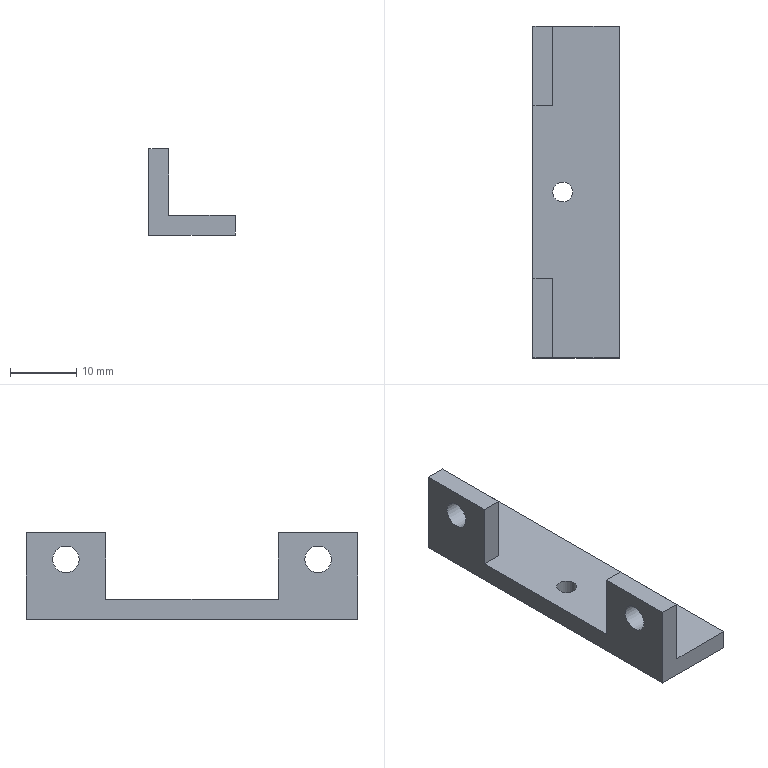Part | STEP file | 1-02 | 1 solid | 15 faces | box 13 x 50 x 13 mm | volume 2573 mm3 | plane 12 | cylinder 3 | commonest cylinder face diameters 4 x2 3 x1
STEP:
#1=CARTESIAN_POINT('',(0.,0.,0.));
#2=DIRECTION('',(0.,0.,1.));
#3=DIRECTION('',(1.,0.,0.));
#4=AXIS2_PLACEMENT_3D('',#1,#2,#3);
#5=CARTESIAN_POINT('',(-6.5,-25.,-3.));
#6=VERTEX_POINT('',#5);
#7=CARTESIAN_POINT('',(6.5,-25.,-3.));
#8=VERTEX_POINT('',#7);
#9=CARTESIAN_POINT('',(-6.5,-25.,-3.));
#10=DIRECTION('',(1.,0.,0.));
#11=VECTOR('',#10,1.);
#12=LINE('',#9,#11);
#13=CARTESIAN_POINT('',(18.5,0.,-3.));
#14=DIRECTION('',(0.,0.,1.));
#15=DIRECTION('',(1.,0.,0.));
#16=AXIS2_PLACEMENT_3D('',#13,#14,#15);
#17=PLANE('',#16);
#18=CARTESIAN_POINT('',(-25.,-25.));
#19=DIRECTION('',(1.,0.));
#20=VECTOR('',#19,1.);
#21=LINE('',#18,#20);
#22=(GEOMETRIC_REPRESENTATION_CONTEXT(2)PARAMETRIC_REPRESENTATION_CONTEXT()REPRESENTATION_CONTEXT('',''));
#23=DEFINITIONAL_REPRESENTATION('',(#21),#22);
#24=PCURVE('',#17,#23);
#25=CARTESIAN_POINT('',(0.,-25.,3.5));
#26=DIRECTION('',(0.,1.,0.));
#27=DIRECTION('',(1.,0.,0.));
#28=AXIS2_PLACEMENT_3D('',#25,#26,#27);
#29=PLANE('',#28);
#30=CARTESIAN_POINT('',(-6.5,6.5));
#31=DIRECTION('',(1.,0.));
#32=VECTOR('',#31,1.);
#33=LINE('',#30,#32);
#34=(GEOMETRIC_REPRESENTATION_CONTEXT(2)PARAMETRIC_REPRESENTATION_CONTEXT()REPRESENTATION_CONTEXT('',''));
#35=DEFINITIONAL_REPRESENTATION('',(#33),#34);
#36=PCURVE('',#29,#35);
#37=SURFACE_CURVE('',#12,(#24,#36),.PCURVE_S1.);
#38=EDGE_CURVE('',#6,#8,#37,.T.);
#39=ORIENTED_EDGE('',*,*,#38,.T.);
#40=CARTESIAN_POINT('',(6.5,25.,-3.));
#41=VERTEX_POINT('',#40);
#42=CARTESIAN_POINT('',(6.5,-25.,-3.));
#43=DIRECTION('',(0.,1.,0.));
#44=VECTOR('',#43,1.);
#45=LINE('',#42,#44);
#46=CARTESIAN_POINT('',(-12.,-25.));
#47=DIRECTION('',(0.,1.));
#48=VECTOR('',#47,1.);
#49=LINE('',#46,#48);
#50=(GEOMETRIC_REPRESENTATION_CONTEXT(2)PARAMETRIC_REPRESENTATION_CONTEXT()REPRESENTATION_CONTEXT('',''));
#51=DEFINITIONAL_REPRESENTATION('',(#49),#50);
#52=PCURVE('',#17,#51);
#53=CARTESIAN_POINT('',(6.5,0.,-1.5));
#54=DIRECTION('',(-1.,0.,0.));
#55=DIRECTION('',(0.,1.,0.));
#56=AXIS2_PLACEMENT_3D('',#53,#54,#55);
#57=PLANE('',#56);
#58=CARTESIAN_POINT('',(-25.,1.5));
#59=DIRECTION('',(1.,0.));
#60=VECTOR('',#59,1.);
#61=LINE('',#58,#60);
#62=(GEOMETRIC_REPRESENTATION_CONTEXT(2)PARAMETRIC_REPRESENTATION_CONTEXT()REPRESENTATION_CONTEXT('',''));
#63=DEFINITIONAL_REPRESENTATION('',(#61),#62);
#64=PCURVE('',#57,#63);
#65=SURFACE_CURVE('',#45,(#52,#64),.PCURVE_S1.);
#66=EDGE_CURVE('',#8,#41,#65,.T.);
#67=ORIENTED_EDGE('',*,*,#66,.T.);
#68=CARTESIAN_POINT('',(-6.5,25.,-3.));
#69=VERTEX_POINT('',#68);
#70=CARTESIAN_POINT('',(6.5,25.,-3.));
#71=DIRECTION('',(-1.,0.,0.));
#72=VECTOR('',#71,1.);
#73=LINE('',#70,#72);
#74=CARTESIAN_POINT('',(-12.,25.));
#75=DIRECTION('',(-1.,0.));
#76=VECTOR('',#75,1.);
#77=LINE('',#74,#76);
#78=(GEOMETRIC_REPRESENTATION_CONTEXT(2)PARAMETRIC_REPRESENTATION_CONTEXT()REPRESENTATION_CONTEXT('',''));
#79=DEFINITIONAL_REPRESENTATION('',(#77),#78);
#80=PCURVE('',#17,#79);
#81=CARTESIAN_POINT('',(0.,25.,3.5));
#82=DIRECTION('',(0.,-1.,0.));
#83=DIRECTION('',(-1.,0.,0.));
#84=AXIS2_PLACEMENT_3D('',#81,#82,#83);
#85=PLANE('',#84);
#86=CARTESIAN_POINT('',(-6.5,6.5));
#87=DIRECTION('',(1.,0.));
#88=VECTOR('',#87,1.);
#89=LINE('',#86,#88);
#90=(GEOMETRIC_REPRESENTATION_CONTEXT(2)PARAMETRIC_REPRESENTATION_CONTEXT()REPRESENTATION_CONTEXT('',''));
#91=DEFINITIONAL_REPRESENTATION('',(#89),#90);
#92=PCURVE('',#85,#91);
#93=SURFACE_CURVE('',#73,(#80,#92),.PCURVE_S1.);
#94=EDGE_CURVE('',#41,#69,#93,.T.);
#95=ORIENTED_EDGE('',*,*,#94,.T.);
#96=CARTESIAN_POINT('',(-6.5,25.,-3.));
#97=DIRECTION('',(0.,-1.,0.));
#98=VECTOR('',#97,1.);
#99=LINE('',#96,#98);
#100=CARTESIAN_POINT('',(-25.,25.));
#101=DIRECTION('',(0.,-1.));
#102=VECTOR('',#101,1.);
#103=LINE('',#100,#102);
#104=(GEOMETRIC_REPRESENTATION_CONTEXT(2)PARAMETRIC_REPRESENTATION_CONTEXT()REPRESENTATION_CONTEXT('',''));
#105=DEFINITIONAL_REPRESENTATION('',(#103),#104);
#106=PCURVE('',#17,#105);
#107=CARTESIAN_POINT('',(-6.5,0.,4.8));
#108=DIRECTION('',(1.,0.,0.));
#109=DIRECTION('',(0.,-1.,0.));
#110=AXIS2_PLACEMENT_3D('',#107,#108,#109);
#111=PLANE('',#110);
#112=CARTESIAN_POINT('',(-25.,7.8));
#113=DIRECTION('',(1.,0.));
#114=VECTOR('',#113,1.);
#115=LINE('',#112,#114);
#116=(GEOMETRIC_REPRESENTATION_CONTEXT(2)PARAMETRIC_REPRESENTATION_CONTEXT()REPRESENTATION_CONTEXT('',''));
#117=DEFINITIONAL_REPRESENTATION('',(#115),#116);
#118=PCURVE('',#111,#117);
#119=SURFACE_CURVE('',#99,(#106,#118),.PCURVE_S1.);
#120=EDGE_CURVE('',#69,#6,#119,.T.);
#121=ORIENTED_EDGE('',*,*,#120,.T.);
#122=EDGE_LOOP('',(#39,#67,#95,#121));
#123=FACE_BOUND('',#122,.F.);
#124=CARTESIAN_POINT('',(-0.5,0.,-3.));
#125=VERTEX_POINT('',#124);
#126=CARTESIAN_POINT('',(-2.,0.,-3.));
#127=DIRECTION('',(0.,0.,-1.));
#128=DIRECTION('',(1.,0.,0.));
#129=AXIS2_PLACEMENT_3D('',#126,#127,#128);
#130=CIRCLE('',#129,1.5);
#131=CARTESIAN_POINT('',(-19.,0.));
#132=CARTESIAN_POINT('',(-19.,-2.598));
#133=CARTESIAN_POINT('',(-21.25,-1.299));
#134=CARTESIAN_POINT('',(-23.5,0.));
#135=CARTESIAN_POINT('',(-21.25,1.299));
#136=CARTESIAN_POINT('',(-19.,2.598));
#137=CARTESIAN_POINT('',(-19.,0.));
#138=(BOUNDED_CURVE()B_SPLINE_CURVE(2,(#131,#132,#133,#134,#135,#136,#137),.UNSPECIFIED.,.T.,.F.)B_SPLINE_CURVE_WITH_KNOTS((1,2,2,2,2,1),(-2.094,0.,2.094,4.189,6.283,8.378),.UNSPECIFIED.)CURVE()GEOMETRIC_REPRESENTATION_ITEM()RATIONAL_B_SPLINE_CURVE((1.,0.5,1.,0.5,1.,0.5,1.))REPRESENTATION_ITEM(''));
#139=(GEOMETRIC_REPRESENTATION_CONTEXT(2)PARAMETRIC_REPRESENTATION_CONTEXT()REPRESENTATION_CONTEXT('',''));
#140=DEFINITIONAL_REPRESENTATION('',(#138),#139);
#141=PCURVE('',#17,#140);
#142=CARTESIAN_POINT('',(-2.,0.,0.));
#143=DIRECTION('',(0.,0.,-1.));
#144=DIRECTION('',(1.,0.,0.));
#145=AXIS2_PLACEMENT_3D('',#142,#143,#144);
#146=CYLINDRICAL_SURFACE('',#145,1.5);
#147=CARTESIAN_POINT('',(0.,3.));
#148=DIRECTION('',(1.,0.));
#149=VECTOR('',#148,1.);
#150=LINE('',#147,#149);
#151=(GEOMETRIC_REPRESENTATION_CONTEXT(2)PARAMETRIC_REPRESENTATION_CONTEXT()REPRESENTATION_CONTEXT('',''));
#152=DEFINITIONAL_REPRESENTATION('',(#150),#151);
#153=PCURVE('',#146,#152);
#154=SURFACE_CURVE('',#130,(#141,#153),.PCURVE_S1.);
#155=EDGE_CURVE('',#125,#125,#154,.T.);
#156=ORIENTED_EDGE('',*,*,#155,.T.);
#157=EDGE_LOOP('',(#156));
#158=FACE_BOUND('',#157,.F.);
#159=ADVANCED_FACE('',(#123,#158),#17,.F.);
#160=CARTESIAN_POINT('',(-3.5,-25.,0.));
#161=VERTEX_POINT('',#160);
#162=CARTESIAN_POINT('',(6.5,-25.,0.));
#163=VERTEX_POINT('',#162);
#164=CARTESIAN_POINT('',(-3.5,-25.,0.));
#165=DIRECTION('',(1.,0.,0.));
#166=VECTOR('',#165,1.);
#167=LINE('',#164,#166);
#168=CARTESIAN_POINT('',(-3.5,3.5));
#169=DIRECTION('',(1.,0.));
#170=VECTOR('',#169,1.);
#171=LINE('',#168,#170);
#172=(GEOMETRIC_REPRESENTATION_CONTEXT(2)PARAMETRIC_REPRESENTATION_CONTEXT()REPRESENTATION_CONTEXT('',''));
#173=DEFINITIONAL_REPRESENTATION('',(#171),#172);
#174=PCURVE('',#29,#173);
#175=CARTESIAN_POINT('',(18.5,0.,0.));
#176=DIRECTION('',(0.,0.,1.));
#177=DIRECTION('',(1.,0.,0.));
#178=AXIS2_PLACEMENT_3D('',#175,#176,#177);
#179=PLANE('',#178);
#180=CARTESIAN_POINT('',(-22.,-25.));
#181=DIRECTION('',(1.,0.));
#182=VECTOR('',#181,1.);
#183=LINE('',#180,#182);
#184=(GEOMETRIC_REPRESENTATION_CONTEXT(2)PARAMETRIC_REPRESENTATION_CONTEXT()REPRESENTATION_CONTEXT('',''));
#185=DEFINITIONAL_REPRESENTATION('',(#183),#184);
#186=PCURVE('',#179,#185);
#187=SURFACE_CURVE('',#167,(#174,#186),.PCURVE_S1.);
#188=EDGE_CURVE('',#161,#163,#187,.T.);
#189=ORIENTED_EDGE('',*,*,#188,.T.);
#190=CARTESIAN_POINT('',(6.5,-25.,0.));
#191=DIRECTION('',(0.,0.,-1.));
#192=VECTOR('',#191,1.);
#193=LINE('',#190,#192);
#194=CARTESIAN_POINT('',(6.5,3.5));
#195=DIRECTION('',(0.,1.));
#196=VECTOR('',#195,1.);
#197=LINE('',#194,#196);
#198=(GEOMETRIC_REPRESENTATION_CONTEXT(2)PARAMETRIC_REPRESENTATION_CONTEXT()REPRESENTATION_CONTEXT('',''));
#199=DEFINITIONAL_REPRESENTATION('',(#197),#198);
#200=PCURVE('',#29,#199);
#201=CARTESIAN_POINT('',(-25.,-1.5));
#202=DIRECTION('',(0.,1.));
#203=VECTOR('',#202,1.);
#204=LINE('',#201,#203);
#205=(GEOMETRIC_REPRESENTATION_CONTEXT(2)PARAMETRIC_REPRESENTATION_CONTEXT()REPRESENTATION_CONTEXT('',''));
#206=DEFINITIONAL_REPRESENTATION('',(#204),#205);
#207=PCURVE('',#57,#206);
#208=SURFACE_CURVE('',#193,(#200,#207),.PCURVE_S1.);
#209=EDGE_CURVE('',#163,#8,#208,.T.);
#210=ORIENTED_EDGE('',*,*,#209,.T.);
#211=ORIENTED_EDGE('',*,*,#38,.F.);
#212=CARTESIAN_POINT('',(-6.5,-25.,10.));
#213=VERTEX_POINT('',#212);
#214=CARTESIAN_POINT('',(-6.5,-25.,10.));
#215=DIRECTION('',(0.,0.,-1.));
#216=VECTOR('',#215,1.);
#217=LINE('',#214,#216);
#218=CARTESIAN_POINT('',(-6.5,-6.5));
#219=DIRECTION('',(0.,1.));
#220=VECTOR('',#219,1.);
#221=LINE('',#218,#220);
#222=(GEOMETRIC_REPRESENTATION_CONTEXT(2)PARAMETRIC_REPRESENTATION_CONTEXT()REPRESENTATION_CONTEXT('',''));
#223=DEFINITIONAL_REPRESENTATION('',(#221),#222);
#224=PCURVE('',#29,#223);
#225=CARTESIAN_POINT('',(25.,-5.2));
#226=DIRECTION('',(0.,1.));
#227=VECTOR('',#226,1.);
#228=LINE('',#225,#227);
#229=(GEOMETRIC_REPRESENTATION_CONTEXT(2)PARAMETRIC_REPRESENTATION_CONTEXT()REPRESENTATION_CONTEXT('',''));
#230=DEFINITIONAL_REPRESENTATION('',(#228),#229);
#231=PCURVE('',#111,#230);
#232=SURFACE_CURVE('',#217,(#224,#231),.PCURVE_S1.);
#233=EDGE_CURVE('',#213,#6,#232,.T.);
#234=ORIENTED_EDGE('',*,*,#233,.F.);
#235=CARTESIAN_POINT('',(-3.5,-25.,10.));
#236=VERTEX_POINT('',#235);
#237=CARTESIAN_POINT('',(-6.5,-25.,10.));
#238=DIRECTION('',(1.,0.,0.));
#239=VECTOR('',#238,1.);
#240=LINE('',#237,#239);
#241=CARTESIAN_POINT('',(-6.5,-6.5));
#242=DIRECTION('',(1.,0.));
#243=VECTOR('',#242,1.);
#244=LINE('',#241,#243);
#245=(GEOMETRIC_REPRESENTATION_CONTEXT(2)PARAMETRIC_REPRESENTATION_CONTEXT()REPRESENTATION_CONTEXT('',''));
#246=DEFINITIONAL_REPRESENTATION('',(#244),#245);
#247=PCURVE('',#29,#246);
#248=CARTESIAN_POINT('',(-5.,-19.,10.));
#249=DIRECTION('',(0.,0.,-1.));
#250=DIRECTION('',(0.,1.,0.));
#251=AXIS2_PLACEMENT_3D('',#248,#249,#250);
#252=PLANE('',#251);
#253=CARTESIAN_POINT('',(-6.,-1.5));
#254=DIRECTION('',(0.,1.));
#255=VECTOR('',#254,1.);
#256=LINE('',#253,#255);
#257=(GEOMETRIC_REPRESENTATION_CONTEXT(2)PARAMETRIC_REPRESENTATION_CONTEXT()REPRESENTATION_CONTEXT('',''));
#258=DEFINITIONAL_REPRESENTATION('',(#256),#257);
#259=PCURVE('',#252,#258);
#260=SURFACE_CURVE('',#240,(#247,#259),.PCURVE_S1.);
#261=EDGE_CURVE('',#213,#236,#260,.T.);
#262=ORIENTED_EDGE('',*,*,#261,.T.);
#263=CARTESIAN_POINT('',(-3.5,-25.,0.));
#264=DIRECTION('',(0.,0.,1.));
#265=VECTOR('',#264,1.);
#266=LINE('',#263,#265);
#267=CARTESIAN_POINT('',(-3.5,3.5));
#268=DIRECTION('',(0.,-1.));
#269=VECTOR('',#268,1.);
#270=LINE('',#267,#269);
#271=(GEOMETRIC_REPRESENTATION_CONTEXT(2)PARAMETRIC_REPRESENTATION_CONTEXT()REPRESENTATION_CONTEXT('',''));
#272=DEFINITIONAL_REPRESENTATION('',(#270),#271);
#273=PCURVE('',#29,#272);
#274=CARTESIAN_POINT('',(-3.5,-19.,6.));
#275=DIRECTION('',(-1.,0.,0.));
#276=DIRECTION('',(0.,-1.,0.));
#277=AXIS2_PLACEMENT_3D('',#274,#275,#276);
#278=PLANE('',#277);
#279=CARTESIAN_POINT('',(6.,-6.));
#280=DIRECTION('',(0.,1.));
#281=VECTOR('',#280,1.);
#282=LINE('',#279,#281);
#283=(GEOMETRIC_REPRESENTATION_CONTEXT(2)PARAMETRIC_REPRESENTATION_CONTEXT()REPRESENTATION_CONTEXT('',''));
#284=DEFINITIONAL_REPRESENTATION('',(#282),#283);
#285=PCURVE('',#278,#284);
#286=SURFACE_CURVE('',#266,(#273,#285),.PCURVE_S1.);
#287=EDGE_CURVE('',#161,#236,#286,.T.);
#288=ORIENTED_EDGE('',*,*,#287,.F.);
#289=EDGE_LOOP('',(#189,#210,#211,#234,#262,#288));
#290=FACE_BOUND('',#289,.F.);
#291=ADVANCED_FACE('',(#290),#29,.F.);
#292=CARTESIAN_POINT('',(6.5,25.,0.));
#293=VERTEX_POINT('',#292);
#294=CARTESIAN_POINT('',(6.5,-25.,0.));
#295=DIRECTION('',(0.,1.,0.));
#296=VECTOR('',#295,1.);
#297=LINE('',#294,#296);
#298=CARTESIAN_POINT('',(-25.,-1.5));
#299=DIRECTION('',(1.,0.));
#300=VECTOR('',#299,1.);
#301=LINE('',#298,#300);
#302=(GEOMETRIC_REPRESENTATION_CONTEXT(2)PARAMETRIC_REPRESENTATION_CONTEXT()REPRESENTATION_CONTEXT('',''));
#303=DEFINITIONAL_REPRESENTATION('',(#301),#302);
#304=PCURVE('',#57,#303);
#305=CARTESIAN_POINT('',(-12.,-25.));
#306=DIRECTION('',(0.,1.));
#307=VECTOR('',#306,1.);
#308=LINE('',#305,#307);
#309=(GEOMETRIC_REPRESENTATION_CONTEXT(2)PARAMETRIC_REPRESENTATION_CONTEXT()REPRESENTATION_CONTEXT('',''));
#310=DEFINITIONAL_REPRESENTATION('',(#308),#309);
#311=PCURVE('',#179,#310);
#312=SURFACE_CURVE('',#297,(#304,#311),.PCURVE_S1.);
#313=EDGE_CURVE('',#163,#293,#312,.T.);
#314=ORIENTED_EDGE('',*,*,#313,.T.);
#315=CARTESIAN_POINT('',(6.5,25.,0.));
#316=DIRECTION('',(0.,0.,-1.));
#317=VECTOR('',#316,1.);
#318=LINE('',#315,#317);
#319=CARTESIAN_POINT('',(25.,-1.5));
#320=DIRECTION('',(0.,1.));
#321=VECTOR('',#320,1.);
#322=LINE('',#319,#321);
#323=(GEOMETRIC_REPRESENTATION_CONTEXT(2)PARAMETRIC_REPRESENTATION_CONTEXT()REPRESENTATION_CONTEXT('',''));
#324=DEFINITIONAL_REPRESENTATION('',(#322),#323);
#325=PCURVE('',#57,#324);
#326=CARTESIAN_POINT('',(-6.5,3.5));
#327=DIRECTION('',(0.,1.));
#328=VECTOR('',#327,1.);
#329=LINE('',#326,#328);
#330=(GEOMETRIC_REPRESENTATION_CONTEXT(2)PARAMETRIC_REPRESENTATION_CONTEXT()REPRESENTATION_CONTEXT('',''));
#331=DEFINITIONAL_REPRESENTATION('',(#329),#330);
#332=PCURVE('',#85,#331);
#333=SURFACE_CURVE('',#318,(#325,#332),.PCURVE_S1.);
#334=EDGE_CURVE('',#293,#41,#333,.T.);
#335=ORIENTED_EDGE('',*,*,#334,.T.);
#336=ORIENTED_EDGE('',*,*,#66,.F.);
#337=ORIENTED_EDGE('',*,*,#209,.F.);
#338=EDGE_LOOP('',(#314,#335,#336,#337));
#339=FACE_BOUND('',#338,.F.);
#340=ADVANCED_FACE('',(#339),#57,.F.);
#341=ORIENTED_EDGE('',*,*,#94,.F.);
#342=ORIENTED_EDGE('',*,*,#334,.F.);
#343=CARTESIAN_POINT('',(-3.5,25.,0.));
#344=VERTEX_POINT('',#343);
#345=CARTESIAN_POINT('',(6.5,25.,0.));
#346=DIRECTION('',(-1.,0.,0.));
#347=VECTOR('',#346,1.);
#348=LINE('',#345,#347);
#349=CARTESIAN_POINT('',(-6.5,3.5));
#350=DIRECTION('',(1.,0.));
#351=VECTOR('',#350,1.);
#352=LINE('',#349,#351);
#353=(GEOMETRIC_REPRESENTATION_CONTEXT(2)PARAMETRIC_REPRESENTATION_CONTEXT()REPRESENTATION_CONTEXT('',''));
#354=DEFINITIONAL_REPRESENTATION('',(#352),#353);
#355=PCURVE('',#85,#354);
#356=CARTESIAN_POINT('',(-12.,25.));
#357=DIRECTION('',(-1.,0.));
#358=VECTOR('',#357,1.);
#359=LINE('',#356,#358);
#360=(GEOMETRIC_REPRESENTATION_CONTEXT(2)PARAMETRIC_REPRESENTATION_CONTEXT()REPRESENTATION_CONTEXT('',''));
#361=DEFINITIONAL_REPRESENTATION('',(#359),#360);
#362=PCURVE('',#179,#361);
#363=SURFACE_CURVE('',#348,(#355,#362),.PCURVE_S1.);
#364=EDGE_CURVE('',#293,#344,#363,.T.);
#365=ORIENTED_EDGE('',*,*,#364,.T.);
#366=CARTESIAN_POINT('',(-3.5,25.,10.));
#367=VERTEX_POINT('',#366);
#368=CARTESIAN_POINT('',(-3.5,25.,10.));
#369=DIRECTION('',(0.,0.,-1.));
#370=VECTOR('',#369,1.);
#371=LINE('',#368,#370);
#372=CARTESIAN_POINT('',(3.5,-6.5));
#373=DIRECTION('',(0.,1.));
#374=VECTOR('',#373,1.);
#375=LINE('',#372,#374);
#376=(GEOMETRIC_REPRESENTATION_CONTEXT(2)PARAMETRIC_REPRESENTATION_CONTEXT()REPRESENTATION_CONTEXT('',''));
#377=DEFINITIONAL_REPRESENTATION('',(#375),#376);
#378=PCURVE('',#85,#377);
#379=CARTESIAN_POINT('',(-3.5,19.,6.));
#380=DIRECTION('',(-1.,0.,0.));
#381=DIRECTION('',(0.,-1.,0.));
#382=AXIS2_PLACEMENT_3D('',#379,#380,#381);
#383=PLANE('',#382);
#384=CARTESIAN_POINT('',(-6.,4.));
#385=DIRECTION('',(0.,-1.));
#386=VECTOR('',#385,1.);
#387=LINE('',#384,#386);
#388=(GEOMETRIC_REPRESENTATION_CONTEXT(2)PARAMETRIC_REPRESENTATION_CONTEXT()REPRESENTATION_CONTEXT('',''));
#389=DEFINITIONAL_REPRESENTATION('',(#387),#388);
#390=PCURVE('',#383,#389);
#391=SURFACE_CURVE('',#371,(#378,#390),.PCURVE_S1.);
#392=EDGE_CURVE('',#367,#344,#391,.T.);
#393=ORIENTED_EDGE('',*,*,#392,.F.);
#394=CARTESIAN_POINT('',(-6.5,25.,10.));
#395=VERTEX_POINT('',#394);
#396=CARTESIAN_POINT('',(-6.5,25.,10.));
#397=DIRECTION('',(1.,0.,0.));
#398=VECTOR('',#397,1.);
#399=LINE('',#396,#398);
#400=CARTESIAN_POINT('',(6.5,-6.5));
#401=DIRECTION('',(-1.,0.));
#402=VECTOR('',#401,1.);
#403=LINE('',#400,#402);
#404=(GEOMETRIC_REPRESENTATION_CONTEXT(2)PARAMETRIC_REPRESENTATION_CONTEXT()REPRESENTATION_CONTEXT('',''));
#405=DEFINITIONAL_REPRESENTATION('',(#403),#404);
#406=PCURVE('',#85,#405);
#407=CARTESIAN_POINT('',(-5.,19.,10.));
#408=DIRECTION('',(0.,0.,-1.));
#409=DIRECTION('',(0.,1.,0.));
#410=AXIS2_PLACEMENT_3D('',#407,#408,#409);
#411=PLANE('',#410);
#412=CARTESIAN_POINT('',(6.,-1.5));
#413=DIRECTION('',(0.,1.));
#414=VECTOR('',#413,1.);
#415=LINE('',#412,#414);
#416=(GEOMETRIC_REPRESENTATION_CONTEXT(2)PARAMETRIC_REPRESENTATION_CONTEXT()REPRESENTATION_CONTEXT('',''));
#417=DEFINITIONAL_REPRESENTATION('',(#415),#416);
#418=PCURVE('',#411,#417);
#419=SURFACE_CURVE('',#399,(#406,#418),.PCURVE_S1.);
#420=EDGE_CURVE('',#395,#367,#419,.T.);
#421=ORIENTED_EDGE('',*,*,#420,.F.);
#422=CARTESIAN_POINT('',(-6.5,25.,-3.));
#423=DIRECTION('',(0.,0.,1.));
#424=VECTOR('',#423,1.);
#425=LINE('',#422,#424);
#426=CARTESIAN_POINT('',(6.5,6.5));
#427=DIRECTION('',(0.,-1.));
#428=VECTOR('',#427,1.);
#429=LINE('',#426,#428);
#430=(GEOMETRIC_REPRESENTATION_CONTEXT(2)PARAMETRIC_REPRESENTATION_CONTEXT()REPRESENTATION_CONTEXT('',''));
#431=DEFINITIONAL_REPRESENTATION('',(#429),#430);
#432=PCURVE('',#85,#431);
#433=CARTESIAN_POINT('',(-25.,7.8));
#434=DIRECTION('',(0.,-1.));
#435=VECTOR('',#434,1.);
#436=LINE('',#433,#435);
#437=(GEOMETRIC_REPRESENTATION_CONTEXT(2)PARAMETRIC_REPRESENTATION_CONTEXT()REPRESENTATION_CONTEXT('',''));
#438=DEFINITIONAL_REPRESENTATION('',(#436),#437);
#439=PCURVE('',#111,#438);
#440=SURFACE_CURVE('',#425,(#432,#439),.PCURVE_S1.);
#441=EDGE_CURVE('',#69,#395,#440,.T.);
#442=ORIENTED_EDGE('',*,*,#441,.F.);
#443=EDGE_LOOP('',(#341,#342,#365,#393,#421,#442));
#444=FACE_BOUND('',#443,.F.);
#445=ADVANCED_FACE('',(#444),#85,.F.);
#446=CARTESIAN_POINT('',(-6.5,13.,0.));
#447=VERTEX_POINT('',#446);
#448=CARTESIAN_POINT('',(-6.5,-13.,0.));
#449=VERTEX_POINT('',#448);
#450=CARTESIAN_POINT('',(-6.5,13.,0.));
#451=DIRECTION('',(0.,-1.,0.));
#452=VECTOR('',#451,1.);
#453=LINE('',#450,#452);
#454=CARTESIAN_POINT('',(-13.,4.8));
#455=DIRECTION('',(1.,0.));
#456=VECTOR('',#455,1.);
#457=LINE('',#454,#456);
#458=(GEOMETRIC_REPRESENTATION_CONTEXT(2)PARAMETRIC_REPRESENTATION_CONTEXT()REPRESENTATION_CONTEXT('',''));
#459=DEFINITIONAL_REPRESENTATION('',(#457),#458);
#460=PCURVE('',#111,#459);
#461=CARTESIAN_POINT('',(-25.,13.));
#462=DIRECTION('',(0.,-1.));
#463=VECTOR('',#462,1.);
#464=LINE('',#461,#463);
#465=(GEOMETRIC_REPRESENTATION_CONTEXT(2)PARAMETRIC_REPRESENTATION_CONTEXT()REPRESENTATION_CONTEXT('',''));
#466=DEFINITIONAL_REPRESENTATION('',(#464),#465);
#467=PCURVE('',#179,#466);
#468=SURFACE_CURVE('',#453,(#460,#467),.PCURVE_S1.);
#469=EDGE_CURVE('',#447,#449,#468,.T.);
#470=ORIENTED_EDGE('',*,*,#469,.T.);
#471=CARTESIAN_POINT('',(-6.5,-13.,10.));
#472=VERTEX_POINT('',#471);
#473=CARTESIAN_POINT('',(-6.5,-13.,10.));
#474=DIRECTION('',(0.,0.,-1.));
#475=VECTOR('',#474,1.);
#476=LINE('',#473,#475);
#477=CARTESIAN_POINT('',(13.,-5.2));
#478=DIRECTION('',(0.,1.));
#479=VECTOR('',#478,1.);
#480=LINE('',#477,#479);
#481=(GEOMETRIC_REPRESENTATION_CONTEXT(2)PARAMETRIC_REPRESENTATION_CONTEXT()REPRESENTATION_CONTEXT('',''));
#482=DEFINITIONAL_REPRESENTATION('',(#480),#481);
#483=PCURVE('',#111,#482);
#484=CARTESIAN_POINT('',(-5.,-13.,5.));
#485=DIRECTION('',(0.,-1.,0.));
#486=DIRECTION('',(0.,0.,-1.));
#487=AXIS2_PLACEMENT_3D('',#484,#485,#486);
#488=PLANE('',#487);
#489=CARTESIAN_POINT('',(-5.,-1.5));
#490=DIRECTION('',(1.,0.));
#491=VECTOR('',#490,1.);
#492=LINE('',#489,#491);
#493=(GEOMETRIC_REPRESENTATION_CONTEXT(2)PARAMETRIC_REPRESENTATION_CONTEXT()REPRESENTATION_CONTEXT('',''));
#494=DEFINITIONAL_REPRESENTATION('',(#492),#493);
#495=PCURVE('',#488,#494);
#496=SURFACE_CURVE('',#476,(#483,#495),.PCURVE_S1.);
#497=EDGE_CURVE('',#472,#449,#496,.T.);
#498=ORIENTED_EDGE('',*,*,#497,.F.);
#499=CARTESIAN_POINT('',(-6.5,-25.,10.));
#500=DIRECTION('',(0.,1.,0.));
#501=VECTOR('',#500,1.);
#502=LINE('',#499,#501);
#503=CARTESIAN_POINT('',(25.,-5.2));
#504=DIRECTION('',(-1.,0.));
#505=VECTOR('',#504,1.);
#506=LINE('',#503,#505);
#507=(GEOMETRIC_REPRESENTATION_CONTEXT(2)PARAMETRIC_REPRESENTATION_CONTEXT()REPRESENTATION_CONTEXT('',''));
#508=DEFINITIONAL_REPRESENTATION('',(#506),#507);
#509=PCURVE('',#111,#508);
#510=CARTESIAN_POINT('',(-6.,-1.5));
#511=DIRECTION('',(1.,0.));
#512=VECTOR('',#511,1.);
#513=LINE('',#510,#512);
#514=(GEOMETRIC_REPRESENTATION_CONTEXT(2)PARAMETRIC_REPRESENTATION_CONTEXT()REPRESENTATION_CONTEXT('',''));
#515=DEFINITIONAL_REPRESENTATION('',(#513),#514);
#516=PCURVE('',#252,#515);
#517=SURFACE_CURVE('',#502,(#509,#516),.PCURVE_S1.);
#518=EDGE_CURVE('',#213,#472,#517,.T.);
#519=ORIENTED_EDGE('',*,*,#518,.F.);
#520=ORIENTED_EDGE('',*,*,#233,.T.);
#521=ORIENTED_EDGE('',*,*,#120,.F.);
#522=ORIENTED_EDGE('',*,*,#441,.T.);
#523=CARTESIAN_POINT('',(-6.5,13.,10.));
#524=VERTEX_POINT('',#523);
#525=CARTESIAN_POINT('',(-6.5,13.,10.));
#526=DIRECTION('',(0.,1.,0.));
#527=VECTOR('',#526,1.);
#528=LINE('',#525,#527);
#529=CARTESIAN_POINT('',(-13.,-5.2));
#530=DIRECTION('',(-1.,0.));
#531=VECTOR('',#530,1.);
#532=LINE('',#529,#531);
#533=(GEOMETRIC_REPRESENTATION_CONTEXT(2)PARAMETRIC_REPRESENTATION_CONTEXT()REPRESENTATION_CONTEXT('',''));
#534=DEFINITIONAL_REPRESENTATION('',(#532),#533);
#535=PCURVE('',#111,#534);
#536=CARTESIAN_POINT('',(-6.,-1.5));
#537=DIRECTION('',(1.,0.));
#538=VECTOR('',#537,1.);
#539=LINE('',#536,#538);
#540=(GEOMETRIC_REPRESENTATION_CONTEXT(2)PARAMETRIC_REPRESENTATION_CONTEXT()REPRESENTATION_CONTEXT('',''));
#541=DEFINITIONAL_REPRESENTATION('',(#539),#540);
#542=PCURVE('',#411,#541);
#543=SURFACE_CURVE('',#528,(#535,#542),.PCURVE_S1.);
#544=EDGE_CURVE('',#524,#395,#543,.T.);
#545=ORIENTED_EDGE('',*,*,#544,.F.);
#546=CARTESIAN_POINT('',(-6.5,13.,0.));
#547=DIRECTION('',(0.,0.,1.));
#548=VECTOR('',#547,1.);
#549=LINE('',#546,#548);
#550=CARTESIAN_POINT('',(-13.,4.8));
#551=DIRECTION('',(0.,-1.));
#552=VECTOR('',#551,1.);
#553=LINE('',#550,#552);
#554=(GEOMETRIC_REPRESENTATION_CONTEXT(2)PARAMETRIC_REPRESENTATION_CONTEXT()REPRESENTATION_CONTEXT('',''));
#555=DEFINITIONAL_REPRESENTATION('',(#553),#554);
#556=PCURVE('',#111,#555);
#557=CARTESIAN_POINT('',(-5.,13.,5.));
#558=DIRECTION('',(0.,1.,0.));
#559=DIRECTION('',(0.,0.,1.));
#560=AXIS2_PLACEMENT_3D('',#557,#558,#559);
#561=PLANE('',#560);
#562=CARTESIAN_POINT('',(-5.,-1.5));
#563=DIRECTION('',(1.,0.));
#564=VECTOR('',#563,1.);
#565=LINE('',#562,#564);
#566=(GEOMETRIC_REPRESENTATION_CONTEXT(2)PARAMETRIC_REPRESENTATION_CONTEXT()REPRESENTATION_CONTEXT('',''));
#567=DEFINITIONAL_REPRESENTATION('',(#565),#566);
#568=PCURVE('',#561,#567);
#569=SURFACE_CURVE('',#549,(#556,#568),.PCURVE_S1.);
#570=EDGE_CURVE('',#447,#524,#569,.T.);
#571=ORIENTED_EDGE('',*,*,#570,.F.);
#572=EDGE_LOOP('',(#470,#498,#519,#520,#521,#522,#545,#571));
#573=FACE_BOUND('',#572,.F.);
#574=CARTESIAN_POINT('',(-6.5,17.,6.));
#575=VERTEX_POINT('',#574);
#576=CARTESIAN_POINT('',(-6.5,19.,6.));
#577=DIRECTION('',(1.,0.,0.));
#578=DIRECTION('',(0.,-1.,0.));
#579=AXIS2_PLACEMENT_3D('',#576,#577,#578);
#580=CIRCLE('',#579,2.);
#581=CARTESIAN_POINT('',(-19.,-1.2));
#582=DIRECTION('',(1.,0.));
#583=AXIS2_PLACEMENT_2D('',#581,#582);
#584=CIRCLE('',#583,2.);
#585=(GEOMETRIC_REPRESENTATION_CONTEXT(2)PARAMETRIC_REPRESENTATION_CONTEXT()REPRESENTATION_CONTEXT('',''));
#586=DEFINITIONAL_REPRESENTATION('',(#584),#585);
#587=PCURVE('',#111,#586);
#588=CARTESIAN_POINT('',(-6.5,19.,6.));
#589=DIRECTION('',(1.,0.,0.));
#590=DIRECTION('',(0.,-1.,0.));
#591=AXIS2_PLACEMENT_3D('',#588,#589,#590);
#592=CYLINDRICAL_SURFACE('',#591,2.);
#593=CARTESIAN_POINT('',(0.,0.));
#594=DIRECTION('',(1.,0.));
#595=VECTOR('',#594,1.);
#596=LINE('',#593,#595);
#597=(GEOMETRIC_REPRESENTATION_CONTEXT(2)PARAMETRIC_REPRESENTATION_CONTEXT()REPRESENTATION_CONTEXT('',''));
#598=DEFINITIONAL_REPRESENTATION('',(#596),#597);
#599=PCURVE('',#592,#598);
#600=SURFACE_CURVE('',#580,(#587,#599),.PCURVE_S1.);
#601=EDGE_CURVE('',#575,#575,#600,.T.);
#602=ORIENTED_EDGE('',*,*,#601,.F.);
#603=EDGE_LOOP('',(#602));
#604=FACE_BOUND('',#603,.F.);
#605=CARTESIAN_POINT('',(-6.5,-21.,6.));
#606=VERTEX_POINT('',#605);
#607=CARTESIAN_POINT('',(-6.5,-19.,6.));
#608=DIRECTION('',(1.,0.,0.));
#609=DIRECTION('',(0.,-1.,0.));
#610=AXIS2_PLACEMENT_3D('',#607,#608,#609);
#611=CIRCLE('',#610,2.);
#612=CARTESIAN_POINT('',(19.,-1.2));
#613=DIRECTION('',(1.,0.));
#614=AXIS2_PLACEMENT_2D('',#612,#613);
#615=CIRCLE('',#614,2.);
#616=(GEOMETRIC_REPRESENTATION_CONTEXT(2)PARAMETRIC_REPRESENTATION_CONTEXT()REPRESENTATION_CONTEXT('',''));
#617=DEFINITIONAL_REPRESENTATION('',(#615),#616);
#618=PCURVE('',#111,#617);
#619=CARTESIAN_POINT('',(-6.5,-19.,6.));
#620=DIRECTION('',(1.,0.,0.));
#621=DIRECTION('',(0.,-1.,0.));
#622=AXIS2_PLACEMENT_3D('',#619,#620,#621);
#623=CYLINDRICAL_SURFACE('',#622,2.);
#624=CARTESIAN_POINT('',(0.,0.));
#625=DIRECTION('',(1.,0.));
#626=VECTOR('',#625,1.);
#627=LINE('',#624,#626);
#628=(GEOMETRIC_REPRESENTATION_CONTEXT(2)PARAMETRIC_REPRESENTATION_CONTEXT()REPRESENTATION_CONTEXT('',''));
#629=DEFINITIONAL_REPRESENTATION('',(#627),#628);
#630=PCURVE('',#623,#629);
#631=SURFACE_CURVE('',#611,(#618,#630),.PCURVE_S1.);
#632=EDGE_CURVE('',#606,#606,#631,.T.);
#633=ORIENTED_EDGE('',*,*,#632,.F.);
#634=EDGE_LOOP('',(#633));
#635=FACE_BOUND('',#634,.F.);
#636=ADVANCED_FACE('',(#573,#604,#635),#111,.F.);
#637=CARTESIAN_POINT('',(-0.5,0.,0.));
#638=VERTEX_POINT('',#637);
#639=CARTESIAN_POINT('',(-2.,0.,0.));
#640=DIRECTION('',(0.,0.,-1.));
#641=DIRECTION('',(1.,0.,0.));
#642=AXIS2_PLACEMENT_3D('',#639,#640,#641);
#643=CIRCLE('',#642,1.5);
#644=CARTESIAN_POINT('',(0.,0.));
#645=DIRECTION('',(1.,0.));
#646=VECTOR('',#645,1.);
#647=LINE('',#644,#646);
#648=(GEOMETRIC_REPRESENTATION_CONTEXT(2)PARAMETRIC_REPRESENTATION_CONTEXT()REPRESENTATION_CONTEXT('',''));
#649=DEFINITIONAL_REPRESENTATION('',(#647),#648);
#650=PCURVE('',#146,#649);
#651=CARTESIAN_POINT('',(-19.,0.));
#652=CARTESIAN_POINT('',(-19.,-2.598));
#653=CARTESIAN_POINT('',(-21.25,-1.299));
#654=CARTESIAN_POINT('',(-23.5,0.));
#655=CARTESIAN_POINT('',(-21.25,1.299));
#656=CARTESIAN_POINT('',(-19.,2.598));
#657=CARTESIAN_POINT('',(-19.,0.));
#658=(BOUNDED_CURVE()B_SPLINE_CURVE(2,(#651,#652,#653,#654,#655,#656,#657),.UNSPECIFIED.,.T.,.F.)B_SPLINE_CURVE_WITH_KNOTS((1,2,2,2,2,1),(-2.094,0.,2.094,4.189,6.283,8.378),.UNSPECIFIED.)CURVE()GEOMETRIC_REPRESENTATION_ITEM()RATIONAL_B_SPLINE_CURVE((1.,0.5,1.,0.5,1.,0.5,1.))REPRESENTATION_ITEM(''));
#659=(GEOMETRIC_REPRESENTATION_CONTEXT(2)PARAMETRIC_REPRESENTATION_CONTEXT()REPRESENTATION_CONTEXT('',''));
#660=DEFINITIONAL_REPRESENTATION('',(#658),#659);
#661=PCURVE('',#179,#660);
#662=SURFACE_CURVE('',#643,(#650,#661),.PCURVE_S1.);
#663=EDGE_CURVE('',#638,#638,#662,.T.);
#664=ORIENTED_EDGE('',*,*,#663,.T.);
#665=CARTESIAN_POINT('',(-0.5,0.,0.));
#666=DIRECTION('',(0.,0.,-1.));
#667=VECTOR('',#666,1.);
#668=LINE('',#665,#667);
#669=CARTESIAN_POINT('',(6.283,0.));
#670=DIRECTION('',(0.,1.));
#671=VECTOR('',#670,1.);
#672=LINE('',#669,#671);
#673=(GEOMETRIC_REPRESENTATION_CONTEXT(2)PARAMETRIC_REPRESENTATION_CONTEXT()REPRESENTATION_CONTEXT('',''));
#674=DEFINITIONAL_REPRESENTATION('',(#672),#673);
#675=PCURVE('',#146,#674);
#676=CARTESIAN_POINT('',(0.,0.));
#677=DIRECTION('',(0.,1.));
#678=VECTOR('',#677,1.);
#679=LINE('',#676,#678);
#680=(GEOMETRIC_REPRESENTATION_CONTEXT(2)PARAMETRIC_REPRESENTATION_CONTEXT()REPRESENTATION_CONTEXT('',''));
#681=DEFINITIONAL_REPRESENTATION('',(#679),#680);
#682=PCURVE('',#146,#681);
#683=SEAM_CURVE('',#668,(#675,#682),.PCURVE_S1.);
#684=EDGE_CURVE('',#638,#125,#683,.T.);
#685=ORIENTED_EDGE('',*,*,#684,.T.);
#686=ORIENTED_EDGE('',*,*,#155,.F.);
#687=ORIENTED_EDGE('',*,*,#684,.F.);
#688=EDGE_LOOP('',(#664,#685,#686,#687));
#689=FACE_BOUND('',#688,.F.);
#690=ADVANCED_FACE('',(#689),#146,.F.);
#691=ORIENTED_EDGE('',*,*,#313,.T.);
#692=ORIENTED_EDGE('',*,*,#364,.T.);
#693=CARTESIAN_POINT('',(-3.5,13.,0.));
#694=VERTEX_POINT('',#693);
#695=CARTESIAN_POINT('',(-3.5,25.,0.));
#696=DIRECTION('',(0.,-1.,0.));
#697=VECTOR('',#696,1.);
#698=LINE('',#695,#697);
#699=CARTESIAN_POINT('',(-22.,25.));
#700=DIRECTION('',(0.,-1.));
#701=VECTOR('',#700,1.);
#702=LINE('',#699,#701);
#703=(GEOMETRIC_REPRESENTATION_CONTEXT(2)PARAMETRIC_REPRESENTATION_CONTEXT()REPRESENTATION_CONTEXT('',''));
#704=DEFINITIONAL_REPRESENTATION('',(#702),#703);
#705=PCURVE('',#179,#704);
#706=CARTESIAN_POINT('',(-6.,-6.));
#707=DIRECTION('',(1.,0.));
#708=VECTOR('',#707,1.);
#709=LINE('',#706,#708);
#710=(GEOMETRIC_REPRESENTATION_CONTEXT(2)PARAMETRIC_REPRESENTATION_CONTEXT()REPRESENTATION_CONTEXT('',''));
#711=DEFINITIONAL_REPRESENTATION('',(#709),#710);
#712=PCURVE('',#383,#711);
#713=SURFACE_CURVE('',#698,(#705,#712),.PCURVE_S1.);
#714=EDGE_CURVE('',#344,#694,#713,.T.);
#715=ORIENTED_EDGE('',*,*,#714,.T.);
#716=CARTESIAN_POINT('',(-6.5,13.,0.));
#717=DIRECTION('',(1.,0.,0.));
#718=VECTOR('',#717,1.);
#719=LINE('',#716,#718);
#720=CARTESIAN_POINT('',(-25.,13.));
#721=DIRECTION('',(1.,0.));
#722=VECTOR('',#721,1.);
#723=LINE('',#720,#722);
#724=(GEOMETRIC_REPRESENTATION_CONTEXT(2)PARAMETRIC_REPRESENTATION_CONTEXT()REPRESENTATION_CONTEXT('',''));
#725=DEFINITIONAL_REPRESENTATION('',(#723),#724);
#726=PCURVE('',#179,#725);
#727=CARTESIAN_POINT('',(-5.,-1.5));
#728=DIRECTION('',(0.,1.));
#729=VECTOR('',#728,1.);
#730=LINE('',#727,#729);
#731=(GEOMETRIC_REPRESENTATION_CONTEXT(2)PARAMETRIC_REPRESENTATION_CONTEXT()REPRESENTATION_CONTEXT('',''));
#732=DEFINITIONAL_REPRESENTATION('',(#730),#731);
#733=PCURVE('',#561,#732);
#734=SURFACE_CURVE('',#719,(#726,#733),.PCURVE_S1.);
#735=EDGE_CURVE('',#447,#694,#734,.T.);
#736=ORIENTED_EDGE('',*,*,#735,.F.);
#737=ORIENTED_EDGE('',*,*,#469,.T.);
#738=CARTESIAN_POINT('',(-3.5,-13.,0.));
#739=VERTEX_POINT('',#738);
#740=CARTESIAN_POINT('',(-6.5,-13.,0.));
#741=DIRECTION('',(1.,0.,0.));
#742=VECTOR('',#741,1.);
#743=LINE('',#740,#742);
#744=CARTESIAN_POINT('',(-25.,-13.));
#745=DIRECTION('',(1.,0.));
#746=VECTOR('',#745,1.);
#747=LINE('',#744,#746);
#748=(GEOMETRIC_REPRESENTATION_CONTEXT(2)PARAMETRIC_REPRESENTATION_CONTEXT()REPRESENTATION_CONTEXT('',''));
#749=DEFINITIONAL_REPRESENTATION('',(#747),#748);
#750=PCURVE('',#179,#749);
#751=CARTESIAN_POINT('',(5.,-1.5));
#752=DIRECTION('',(0.,1.));
#753=VECTOR('',#752,1.);
#754=LINE('',#751,#753);
#755=(GEOMETRIC_REPRESENTATION_CONTEXT(2)PARAMETRIC_REPRESENTATION_CONTEXT()REPRESENTATION_CONTEXT('',''));
#756=DEFINITIONAL_REPRESENTATION('',(#754),#755);
#757=PCURVE('',#488,#756);
#758=SURFACE_CURVE('',#743,(#750,#757),.PCURVE_S1.);
#759=EDGE_CURVE('',#449,#739,#758,.T.);
#760=ORIENTED_EDGE('',*,*,#759,.T.);
#761=CARTESIAN_POINT('',(-3.5,-13.,0.));
#762=DIRECTION('',(0.,-1.,0.));
#763=VECTOR('',#762,1.);
#764=LINE('',#761,#763);
#765=CARTESIAN_POINT('',(-22.,-13.));
#766=DIRECTION('',(0.,-1.));
#767=VECTOR('',#766,1.);
#768=LINE('',#765,#767);
#769=(GEOMETRIC_REPRESENTATION_CONTEXT(2)PARAMETRIC_REPRESENTATION_CONTEXT()REPRESENTATION_CONTEXT('',''));
#770=DEFINITIONAL_REPRESENTATION('',(#768),#769);
#771=PCURVE('',#179,#770);
#772=CARTESIAN_POINT('',(-6.,-6.));
#773=DIRECTION('',(1.,0.));
#774=VECTOR('',#773,1.);
#775=LINE('',#772,#774);
#776=(GEOMETRIC_REPRESENTATION_CONTEXT(2)PARAMETRIC_REPRESENTATION_CONTEXT()REPRESENTATION_CONTEXT('',''));
#777=DEFINITIONAL_REPRESENTATION('',(#775),#776);
#778=PCURVE('',#278,#777);
#779=SURFACE_CURVE('',#764,(#771,#778),.PCURVE_S1.);
#780=EDGE_CURVE('',#739,#161,#779,.T.);
#781=ORIENTED_EDGE('',*,*,#780,.T.);
#782=ORIENTED_EDGE('',*,*,#188,.T.);
#783=EDGE_LOOP('',(#691,#692,#715,#736,#737,#760,#781,#782));
#784=FACE_BOUND('',#783,.T.);
#785=ORIENTED_EDGE('',*,*,#663,.T.);
#786=EDGE_LOOP('',(#785));
#787=FACE_BOUND('',#786,.T.);
#788=ADVANCED_FACE('',(#784,#787),#179,.T.);
#789=ORIENTED_EDGE('',*,*,#287,.T.);
#790=CARTESIAN_POINT('',(-3.5,-13.,10.));
#791=VERTEX_POINT('',#790);
#792=CARTESIAN_POINT('',(-3.5,-25.,10.));
#793=DIRECTION('',(0.,1.,0.));
#794=VECTOR('',#793,1.);
#795=LINE('',#792,#794);
#796=CARTESIAN_POINT('',(6.,4.));
#797=DIRECTION('',(-1.,0.));
#798=VECTOR('',#797,1.);
#799=LINE('',#796,#798);
#800=(GEOMETRIC_REPRESENTATION_CONTEXT(2)PARAMETRIC_REPRESENTATION_CONTEXT()REPRESENTATION_CONTEXT('',''));
#801=DEFINITIONAL_REPRESENTATION('',(#799),#800);
#802=PCURVE('',#278,#801);
#803=CARTESIAN_POINT('',(-6.,1.5));
#804=DIRECTION('',(1.,0.));
#805=VECTOR('',#804,1.);
#806=LINE('',#803,#805);
#807=(GEOMETRIC_REPRESENTATION_CONTEXT(2)PARAMETRIC_REPRESENTATION_CONTEXT()REPRESENTATION_CONTEXT('',''));
#808=DEFINITIONAL_REPRESENTATION('',(#806),#807);
#809=PCURVE('',#252,#808);
#810=SURFACE_CURVE('',#795,(#802,#809),.PCURVE_S1.);
#811=EDGE_CURVE('',#236,#791,#810,.T.);
#812=ORIENTED_EDGE('',*,*,#811,.T.);
#813=CARTESIAN_POINT('',(-3.5,-13.,10.));
#814=DIRECTION('',(0.,0.,-1.));
#815=VECTOR('',#814,1.);
#816=LINE('',#813,#815);
#817=CARTESIAN_POINT('',(-6.,4.));
#818=DIRECTION('',(0.,-1.));
#819=VECTOR('',#818,1.);
#820=LINE('',#817,#819);
#821=(GEOMETRIC_REPRESENTATION_CONTEXT(2)PARAMETRIC_REPRESENTATION_CONTEXT()REPRESENTATION_CONTEXT('',''));
#822=DEFINITIONAL_REPRESENTATION('',(#820),#821);
#823=PCURVE('',#278,#822);
#824=CARTESIAN_POINT('',(-5.,1.5));
#825=DIRECTION('',(1.,0.));
#826=VECTOR('',#825,1.);
#827=LINE('',#824,#826);
#828=(GEOMETRIC_REPRESENTATION_CONTEXT(2)PARAMETRIC_REPRESENTATION_CONTEXT()REPRESENTATION_CONTEXT('',''));
#829=DEFINITIONAL_REPRESENTATION('',(#827),#828);
#830=PCURVE('',#488,#829);
#831=SURFACE_CURVE('',#816,(#823,#830),.PCURVE_S1.);
#832=EDGE_CURVE('',#791,#739,#831,.T.);
#833=ORIENTED_EDGE('',*,*,#832,.T.);
#834=ORIENTED_EDGE('',*,*,#780,.T.);
#835=EDGE_LOOP('',(#789,#812,#833,#834));
#836=FACE_BOUND('',#835,.F.);
#837=CARTESIAN_POINT('',(-3.5,-21.,6.));
#838=VERTEX_POINT('',#837);
#839=CARTESIAN_POINT('',(-3.5,-19.,6.));
#840=DIRECTION('',(1.,0.,0.));
#841=DIRECTION('',(0.,-1.,0.));
#842=AXIS2_PLACEMENT_3D('',#839,#840,#841);
#843=CIRCLE('',#842,2.);
#844=CARTESIAN_POINT('',(2.,0.));
#845=CARTESIAN_POINT('',(2.,-3.464));
#846=CARTESIAN_POINT('',(-1.,-1.732));
#847=CARTESIAN_POINT('',(-4.,0.));
#848=CARTESIAN_POINT('',(-1.,1.732));
#849=CARTESIAN_POINT('',(2.,3.464));
#850=CARTESIAN_POINT('',(2.,0.));
#851=(BOUNDED_CURVE()B_SPLINE_CURVE(2,(#844,#845,#846,#847,#848,#849,#850),.UNSPECIFIED.,.T.,.F.)B_SPLINE_CURVE_WITH_KNOTS((1,2,2,2,2,1),(-2.094,0.,2.094,4.189,6.283,8.378),.UNSPECIFIED.)CURVE()GEOMETRIC_REPRESENTATION_ITEM()RATIONAL_B_SPLINE_CURVE((1.,0.5,1.,0.5,1.,0.5,1.))REPRESENTATION_ITEM(''));
#852=(GEOMETRIC_REPRESENTATION_CONTEXT(2)PARAMETRIC_REPRESENTATION_CONTEXT()REPRESENTATION_CONTEXT('',''));
#853=DEFINITIONAL_REPRESENTATION('',(#851),#852);
#854=PCURVE('',#278,#853);
#855=CARTESIAN_POINT('',(0.,3.));
#856=DIRECTION('',(1.,0.));
#857=VECTOR('',#856,1.);
#858=LINE('',#855,#857);
#859=(GEOMETRIC_REPRESENTATION_CONTEXT(2)PARAMETRIC_REPRESENTATION_CONTEXT()REPRESENTATION_CONTEXT('',''));
#860=DEFINITIONAL_REPRESENTATION('',(#858),#859);
#861=PCURVE('',#623,#860);
#862=SURFACE_CURVE('',#843,(#854,#861),.PCURVE_S1.);
#863=EDGE_CURVE('',#838,#838,#862,.T.);
#864=ORIENTED_EDGE('',*,*,#863,.T.);
#865=EDGE_LOOP('',(#864));
#866=FACE_BOUND('',#865,.F.);
#867=ADVANCED_FACE('',(#836,#866),#278,.F.);
#868=ORIENTED_EDGE('',*,*,#518,.T.);
#869=CARTESIAN_POINT('',(-6.5,-13.,10.));
#870=DIRECTION('',(1.,0.,0.));
#871=VECTOR('',#870,1.);
#872=LINE('',#869,#871);
#873=CARTESIAN_POINT('',(6.,-1.5));
#874=DIRECTION('',(0.,1.));
#875=VECTOR('',#874,1.);
#876=LINE('',#873,#875);
#877=(GEOMETRIC_REPRESENTATION_CONTEXT(2)PARAMETRIC_REPRESENTATION_CONTEXT()REPRESENTATION_CONTEXT('',''));
#878=DEFINITIONAL_REPRESENTATION('',(#876),#877);
#879=PCURVE('',#252,#878);
#880=CARTESIAN_POINT('',(-5.,-1.5));
#881=DIRECTION('',(0.,1.));
#882=VECTOR('',#881,1.);
#883=LINE('',#880,#882);
#884=(GEOMETRIC_REPRESENTATION_CONTEXT(2)PARAMETRIC_REPRESENTATION_CONTEXT()REPRESENTATION_CONTEXT('',''));
#885=DEFINITIONAL_REPRESENTATION('',(#883),#884);
#886=PCURVE('',#488,#885);
#887=SURFACE_CURVE('',#872,(#879,#886),.PCURVE_S1.);
#888=EDGE_CURVE('',#472,#791,#887,.T.);
#889=ORIENTED_EDGE('',*,*,#888,.T.);
#890=ORIENTED_EDGE('',*,*,#811,.F.);
#891=ORIENTED_EDGE('',*,*,#261,.F.);
#892=EDGE_LOOP('',(#868,#889,#890,#891));
#893=FACE_BOUND('',#892,.F.);
#894=ADVANCED_FACE('',(#893),#252,.F.);
#895=ORIENTED_EDGE('',*,*,#714,.T.);
#896=CARTESIAN_POINT('',(-3.5,13.,10.));
#897=VERTEX_POINT('',#896);
#898=CARTESIAN_POINT('',(-3.5,13.,0.));
#899=DIRECTION('',(0.,0.,1.));
#900=VECTOR('',#899,1.);
#901=LINE('',#898,#900);
#902=CARTESIAN_POINT('',(6.,-6.));
#903=DIRECTION('',(0.,1.));
#904=VECTOR('',#903,1.);
#905=LINE('',#902,#904);
#906=(GEOMETRIC_REPRESENTATION_CONTEXT(2)PARAMETRIC_REPRESENTATION_CONTEXT()REPRESENTATION_CONTEXT('',''));
#907=DEFINITIONAL_REPRESENTATION('',(#905),#906);
#908=PCURVE('',#383,#907);
#909=CARTESIAN_POINT('',(-5.,1.5));
#910=DIRECTION('',(1.,0.));
#911=VECTOR('',#910,1.);
#912=LINE('',#909,#911);
#913=(GEOMETRIC_REPRESENTATION_CONTEXT(2)PARAMETRIC_REPRESENTATION_CONTEXT()REPRESENTATION_CONTEXT('',''));
#914=DEFINITIONAL_REPRESENTATION('',(#912),#913);
#915=PCURVE('',#561,#914);
#916=SURFACE_CURVE('',#901,(#908,#915),.PCURVE_S1.);
#917=EDGE_CURVE('',#694,#897,#916,.T.);
#918=ORIENTED_EDGE('',*,*,#917,.T.);
#919=CARTESIAN_POINT('',(-3.5,13.,10.));
#920=DIRECTION('',(0.,1.,0.));
#921=VECTOR('',#920,1.);
#922=LINE('',#919,#921);
#923=CARTESIAN_POINT('',(6.,4.));
#924=DIRECTION('',(-1.,0.));
#925=VECTOR('',#924,1.);
#926=LINE('',#923,#925);
#927=(GEOMETRIC_REPRESENTATION_CONTEXT(2)PARAMETRIC_REPRESENTATION_CONTEXT()REPRESENTATION_CONTEXT('',''));
#928=DEFINITIONAL_REPRESENTATION('',(#926),#927);
#929=PCURVE('',#383,#928);
#930=CARTESIAN_POINT('',(-6.,1.5));
#931=DIRECTION('',(1.,0.));
#932=VECTOR('',#931,1.);
#933=LINE('',#930,#932);
#934=(GEOMETRIC_REPRESENTATION_CONTEXT(2)PARAMETRIC_REPRESENTATION_CONTEXT()REPRESENTATION_CONTEXT('',''));
#935=DEFINITIONAL_REPRESENTATION('',(#933),#934);
#936=PCURVE('',#411,#935);
#937=SURFACE_CURVE('',#922,(#929,#936),.PCURVE_S1.);
#938=EDGE_CURVE('',#897,#367,#937,.T.);
#939=ORIENTED_EDGE('',*,*,#938,.T.);
#940=ORIENTED_EDGE('',*,*,#392,.T.);
#941=EDGE_LOOP('',(#895,#918,#939,#940));
#942=FACE_BOUND('',#941,.F.);
#943=CARTESIAN_POINT('',(-3.5,17.,6.));
#944=VERTEX_POINT('',#943);
#945=CARTESIAN_POINT('',(-3.5,19.,6.));
#946=DIRECTION('',(1.,0.,0.));
#947=DIRECTION('',(0.,-1.,0.));
#948=AXIS2_PLACEMENT_3D('',#945,#946,#947);
#949=CIRCLE('',#948,2.);
#950=CARTESIAN_POINT('',(2.,0.));
#951=CARTESIAN_POINT('',(2.,-3.464));
#952=CARTESIAN_POINT('',(-1.,-1.732));
#953=CARTESIAN_POINT('',(-4.,0.));
#954=CARTESIAN_POINT('',(-1.,1.732));
#955=CARTESIAN_POINT('',(2.,3.464));
#956=CARTESIAN_POINT('',(2.,0.));
#957=(BOUNDED_CURVE()B_SPLINE_CURVE(2,(#950,#951,#952,#953,#954,#955,#956),.UNSPECIFIED.,.T.,.F.)B_SPLINE_CURVE_WITH_KNOTS((1,2,2,2,2,1),(-2.094,0.,2.094,4.189,6.283,8.378),.UNSPECIFIED.)CURVE()GEOMETRIC_REPRESENTATION_ITEM()RATIONAL_B_SPLINE_CURVE((1.,0.5,1.,0.5,1.,0.5,1.))REPRESENTATION_ITEM(''));
#958=(GEOMETRIC_REPRESENTATION_CONTEXT(2)PARAMETRIC_REPRESENTATION_CONTEXT()REPRESENTATION_CONTEXT('',''));
#959=DEFINITIONAL_REPRESENTATION('',(#957),#958);
#960=PCURVE('',#383,#959);
#961=CARTESIAN_POINT('',(0.,3.));
#962=DIRECTION('',(1.,0.));
#963=VECTOR('',#962,1.);
#964=LINE('',#961,#963);
#965=(GEOMETRIC_REPRESENTATION_CONTEXT(2)PARAMETRIC_REPRESENTATION_CONTEXT()REPRESENTATION_CONTEXT('',''));
#966=DEFINITIONAL_REPRESENTATION('',(#964),#965);
#967=PCURVE('',#592,#966);
#968=SURFACE_CURVE('',#949,(#960,#967),.PCURVE_S1.);
#969=EDGE_CURVE('',#944,#944,#968,.T.);
#970=ORIENTED_EDGE('',*,*,#969,.T.);
#971=EDGE_LOOP('',(#970));
#972=FACE_BOUND('',#971,.F.);
#973=ADVANCED_FACE('',(#942,#972),#383,.F.);
#974=ORIENTED_EDGE('',*,*,#570,.T.);
#975=CARTESIAN_POINT('',(-6.5,13.,10.));
#976=DIRECTION('',(1.,0.,0.));
#977=VECTOR('',#976,1.);
#978=LINE('',#975,#977);
#979=CARTESIAN_POINT('',(5.,-1.5));
#980=DIRECTION('',(0.,1.));
#981=VECTOR('',#980,1.);
#982=LINE('',#979,#981);
#983=(GEOMETRIC_REPRESENTATION_CONTEXT(2)PARAMETRIC_REPRESENTATION_CONTEXT()REPRESENTATION_CONTEXT('',''));
#984=DEFINITIONAL_REPRESENTATION('',(#982),#983);
#985=PCURVE('',#561,#984);
#986=CARTESIAN_POINT('',(-6.,-1.5));
#987=DIRECTION('',(0.,1.));
#988=VECTOR('',#987,1.);
#989=LINE('',#986,#988);
#990=(GEOMETRIC_REPRESENTATION_CONTEXT(2)PARAMETRIC_REPRESENTATION_CONTEXT()REPRESENTATION_CONTEXT('',''));
#991=DEFINITIONAL_REPRESENTATION('',(#989),#990);
#992=PCURVE('',#411,#991);
#993=SURFACE_CURVE('',#978,(#985,#992),.PCURVE_S1.);
#994=EDGE_CURVE('',#524,#897,#993,.T.);
#995=ORIENTED_EDGE('',*,*,#994,.T.);
#996=ORIENTED_EDGE('',*,*,#917,.F.);
#997=ORIENTED_EDGE('',*,*,#735,.F.);
#998=EDGE_LOOP('',(#974,#995,#996,#997));
#999=FACE_BOUND('',#998,.F.);
#1000=ADVANCED_FACE('',(#999),#561,.F.);
#1001=ORIENTED_EDGE('',*,*,#497,.T.);
#1002=ORIENTED_EDGE('',*,*,#759,.T.);
#1003=ORIENTED_EDGE('',*,*,#832,.F.);
#1004=ORIENTED_EDGE('',*,*,#888,.F.);
#1005=EDGE_LOOP('',(#1001,#1002,#1003,#1004));
#1006=FACE_BOUND('',#1005,.F.);
#1007=ADVANCED_FACE('',(#1006),#488,.F.);
#1008=ORIENTED_EDGE('',*,*,#544,.T.);
#1009=ORIENTED_EDGE('',*,*,#420,.T.);
#1010=ORIENTED_EDGE('',*,*,#938,.F.);
#1011=ORIENTED_EDGE('',*,*,#994,.F.);
#1012=EDGE_LOOP('',(#1008,#1009,#1010,#1011));
#1013=FACE_BOUND('',#1012,.F.);
#1014=ADVANCED_FACE('',(#1013),#411,.F.);
#1015=ORIENTED_EDGE('',*,*,#601,.T.);
#1016=CARTESIAN_POINT('',(-6.5,17.,6.));
#1017=DIRECTION('',(1.,0.,0.));
#1018=VECTOR('',#1017,1.);
#1019=LINE('',#1016,#1018);
#1020=CARTESIAN_POINT('',(6.283,0.));
#1021=DIRECTION('',(0.,1.));
#1022=VECTOR('',#1021,1.);
#1023=LINE('',#1020,#1022);
#1024=(GEOMETRIC_REPRESENTATION_CONTEXT(2)PARAMETRIC_REPRESENTATION_CONTEXT()REPRESENTATION_CONTEXT('',''));
#1025=DEFINITIONAL_REPRESENTATION('',(#1023),#1024);
#1026=PCURVE('',#592,#1025);
#1027=CARTESIAN_POINT('',(0.,0.));
#1028=DIRECTION('',(0.,1.));
#1029=VECTOR('',#1028,1.);
#1030=LINE('',#1027,#1029);
#1031=(GEOMETRIC_REPRESENTATION_CONTEXT(2)PARAMETRIC_REPRESENTATION_CONTEXT()REPRESENTATION_CONTEXT('',''));
#1032=DEFINITIONAL_REPRESENTATION('',(#1030),#1031);
#1033=PCURVE('',#592,#1032);
#1034=SEAM_CURVE('',#1019,(#1026,#1033),.PCURVE_S1.);
#1035=EDGE_CURVE('',#575,#944,#1034,.T.);
#1036=ORIENTED_EDGE('',*,*,#1035,.T.);
#1037=ORIENTED_EDGE('',*,*,#969,.F.);
#1038=ORIENTED_EDGE('',*,*,#1035,.F.);
#1039=EDGE_LOOP('',(#1015,#1036,#1037,#1038));
#1040=FACE_BOUND('',#1039,.F.);
#1041=ADVANCED_FACE('',(#1040),#592,.F.);
#1042=ORIENTED_EDGE('',*,*,#632,.T.);
#1043=CARTESIAN_POINT('',(-6.5,-21.,6.));
#1044=DIRECTION('',(1.,0.,0.));
#1045=VECTOR('',#1044,1.);
#1046=LINE('',#1043,#1045);
#1047=CARTESIAN_POINT('',(6.283,0.));
#1048=DIRECTION('',(0.,1.));
#1049=VECTOR('',#1048,1.);
#1050=LINE('',#1047,#1049);
#1051=(GEOMETRIC_REPRESENTATION_CONTEXT(2)PARAMETRIC_REPRESENTATION_CONTEXT()REPRESENTATION_CONTEXT('',''));
#1052=DEFINITIONAL_REPRESENTATION('',(#1050),#1051);
#1053=PCURVE('',#623,#1052);
#1054=CARTESIAN_POINT('',(0.,0.));
#1055=DIRECTION('',(0.,1.));
#1056=VECTOR('',#1055,1.);
#1057=LINE('',#1054,#1056);
#1058=(GEOMETRIC_REPRESENTATION_CONTEXT(2)PARAMETRIC_REPRESENTATION_CONTEXT()REPRESENTATION_CONTEXT('',''));
#1059=DEFINITIONAL_REPRESENTATION('',(#1057),#1058);
#1060=PCURVE('',#623,#1059);
#1061=SEAM_CURVE('',#1046,(#1053,#1060),.PCURVE_S1.);
#1062=EDGE_CURVE('',#606,#838,#1061,.T.);
#1063=ORIENTED_EDGE('',*,*,#1062,.T.);
#1064=ORIENTED_EDGE('',*,*,#863,.F.);
#1065=ORIENTED_EDGE('',*,*,#1062,.F.);
#1066=EDGE_LOOP('',(#1042,#1063,#1064,#1065));
#1067=FACE_BOUND('',#1066,.F.);
#1068=ADVANCED_FACE('',(#1067),#623,.F.);
#1069=CLOSED_SHELL('',(#159,#291,#340,#445,#636,#690,#788,#867,#894,#973,#1000,#1007,#1014,#1041,#1068));
#1070=MANIFOLD_SOLID_BREP('',#1069);
#1071=(LENGTH_UNIT()NAMED_UNIT(*)SI_UNIT(.MILLI.,.METRE.));
#1072=UNCERTAINTY_MEASURE_WITH_UNIT(LENGTH_MEASURE(0.0000001),#1071,'','');
#1073=(NAMED_UNIT(*)PLANE_ANGLE_UNIT()SI_UNIT($,.RADIAN.));
#1074=(NAMED_UNIT(*)SI_UNIT($,.STERADIAN.)SOLID_ANGLE_UNIT());
#1075=(GEOMETRIC_REPRESENTATION_CONTEXT(3)GLOBAL_UNCERTAINTY_ASSIGNED_CONTEXT((#1072))GLOBAL_UNIT_ASSIGNED_CONTEXT((#1071,#1073,#1074))REPRESENTATION_CONTEXT('',''));
#1076=ADVANCED_BREP_SHAPE_REPRESENTATION('',(#4,#1070),#1075);